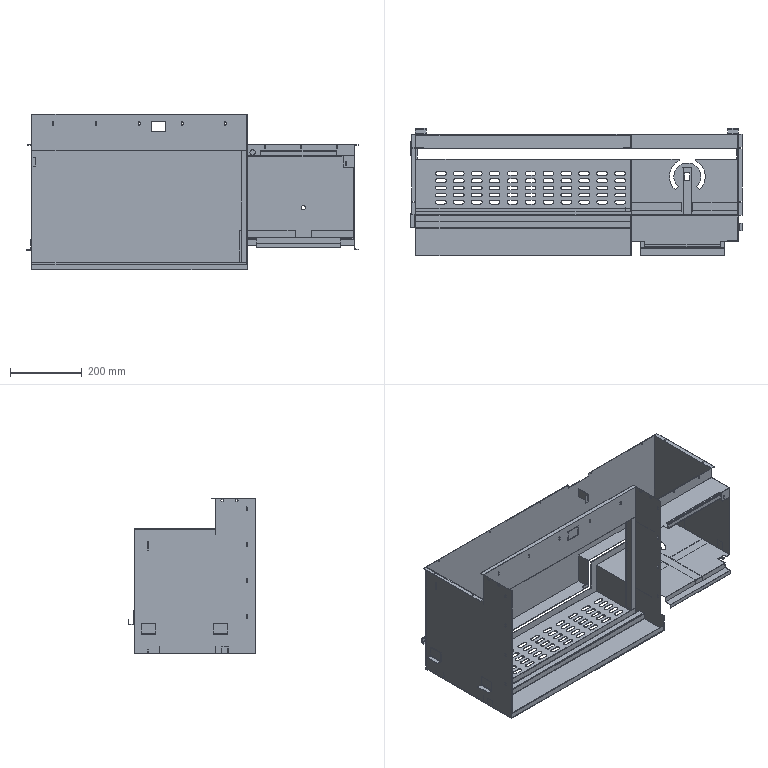Part | STEP file | Transparent screen built-in cover plate 001 | 17 solids | 760 faces | box 926 x 355 x 435 mm | volume 1573889 mm3 | plane 452 | cylinder 304 | cone 4 | commonest cylinder face diameters 10 x165 4 x54 3.5 x22 6 x20 3 x15 2.5 x14